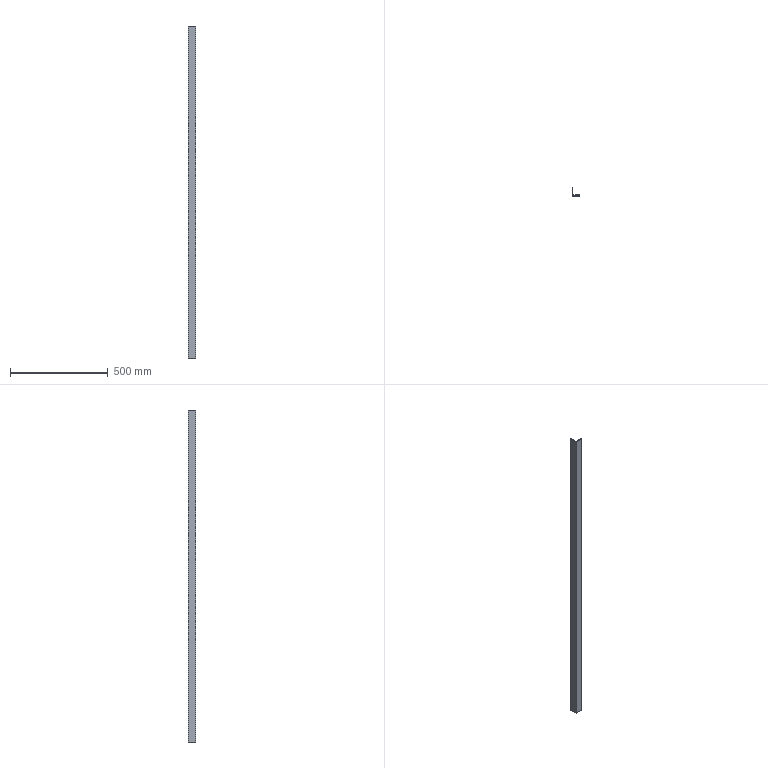Part | SolidWorks | features Extrusion 1 | 1 solid | 11 faces | box 40 x 40 x 1700 mm | volume 524623 mm3 | plane 8 | cylinder 3 | commonest cylinder face diameters 2.667 x2 10 x1
STEP:
#1=CARTESIAN_POINT('',(9.,4.,0.));
#2=VERTEX_POINT('',#1);
#3=CARTESIAN_POINT('',(4.,9.,0.));
#4=VERTEX_POINT('',#3);
#5=CARTESIAN_POINT('',(9.,9.,0.));
#6=DIRECTION('',(0.,0.,-1.));
#7=DIRECTION('',(-1.,0.,0.));
#8=AXIS2_PLACEMENT_3D('',#5,#6,#7);
#9=CIRCLE('',#8,5.);
#10=EDGE_CURVE('',#2,#4,#9,.T.);
#11=ORIENTED_EDGE('',*,*,#10,.T.);
#12=CARTESIAN_POINT('',(4.,9.,1700.));
#13=VERTEX_POINT('',#12);
#14=CARTESIAN_POINT('',(4.,9.,1700.));
#15=DIRECTION('',(0.,0.,-1.));
#16=VECTOR('',#15,1000.);
#17=LINE('',#14,#16);
#18=EDGE_CURVE('',#13,#4,#17,.T.);
#19=ORIENTED_EDGE('',*,*,#18,.F.);
#20=CARTESIAN_POINT('',(9.,4.,1700.));
#21=VERTEX_POINT('',#20);
#22=CARTESIAN_POINT('',(9.,9.,1700.));
#23=DIRECTION('',(0.,0.,-1.));
#24=DIRECTION('',(-1.,0.,0.));
#25=AXIS2_PLACEMENT_3D('',#22,#23,#24);
#26=CIRCLE('',#25,5.);
#27=EDGE_CURVE('',#21,#13,#26,.T.);
#28=ORIENTED_EDGE('',*,*,#27,.F.);
#29=CARTESIAN_POINT('',(9.,4.,1700.));
#30=DIRECTION('',(0.,0.,-1.));
#31=VECTOR('',#30,1000.);
#32=LINE('',#29,#31);
#33=EDGE_CURVE('',#21,#2,#32,.T.);
#34=ORIENTED_EDGE('',*,*,#33,.T.);
#35=EDGE_LOOP('',(#11,#19,#28,#34));
#36=FACE_OUTER_BOUND('',#35,.T.);
#37=CARTESIAN_POINT('',(9.,9.,1700.));
#38=DIRECTION('',(0.,0.,-1.));
#39=DIRECTION('',(-1.,0.,0.));
#40=AXIS2_PLACEMENT_3D('',#37,#38,#39);
#41=CYLINDRICAL_SURFACE('',#40,5.);
#42=ADVANCED_FACE('',(#36),#41,.F.);
#43=CARTESIAN_POINT('',(4.,38.667,0.));
#44=VERTEX_POINT('',#43);
#45=CARTESIAN_POINT('',(4.,38.667,0.));
#46=DIRECTION('',(0.,-1.,0.));
#47=VECTOR('',#46,1000.);
#48=LINE('',#45,#47);
#49=EDGE_CURVE('',#44,#4,#48,.T.);
#50=ORIENTED_EDGE('',*,*,#49,.F.);
#51=CARTESIAN_POINT('',(4.,38.667,1700.));
#52=VERTEX_POINT('',#51);
#53=CARTESIAN_POINT('',(4.,38.667,1700.));
#54=DIRECTION('',(0.,0.,-1.));
#55=VECTOR('',#54,1000.);
#56=LINE('',#53,#55);
#57=EDGE_CURVE('',#52,#44,#56,.T.);
#58=ORIENTED_EDGE('',*,*,#57,.F.);
#59=CARTESIAN_POINT('',(4.,38.667,1700.));
#60=DIRECTION('',(0.,-1.,0.));
#61=VECTOR('',#60,1000.);
#62=LINE('',#59,#61);
#63=EDGE_CURVE('',#52,#13,#62,.T.);
#64=ORIENTED_EDGE('',*,*,#63,.T.);
#65=ORIENTED_EDGE('',*,*,#18,.T.);
#66=EDGE_LOOP('',(#50,#58,#64,#65));
#67=FACE_OUTER_BOUND('',#66,.T.);
#68=CARTESIAN_POINT('',(4.,38.667,1700.));
#69=DIRECTION('',(1.,0.,0.));
#70=DIRECTION('',(0.,1.,0.));
#71=AXIS2_PLACEMENT_3D('',#68,#69,#70);
#72=PLANE('',#71);
#73=ADVANCED_FACE('',(#67),#72,.T.);
#74=CARTESIAN_POINT('',(2.667,40.,0.));
#75=VERTEX_POINT('',#74);
#76=CARTESIAN_POINT('',(2.667,38.667,0.));
#77=DIRECTION('',(0.,0.,-1.));
#78=DIRECTION('',(-1.,0.,0.));
#79=AXIS2_PLACEMENT_3D('',#76,#77,#78);
#80=CIRCLE('',#79,1.333);
#81=EDGE_CURVE('',#75,#44,#80,.T.);
#82=ORIENTED_EDGE('',*,*,#81,.F.);
#83=CARTESIAN_POINT('',(2.667,40.,1700.));
#84=VERTEX_POINT('',#83);
#85=CARTESIAN_POINT('',(2.667,40.,1700.));
#86=DIRECTION('',(0.,0.,-1.));
#87=VECTOR('',#86,1000.);
#88=LINE('',#85,#87);
#89=EDGE_CURVE('',#84,#75,#88,.T.);
#90=ORIENTED_EDGE('',*,*,#89,.F.);
#91=CARTESIAN_POINT('',(2.667,38.667,1700.));
#92=DIRECTION('',(0.,0.,-1.));
#93=DIRECTION('',(-1.,0.,0.));
#94=AXIS2_PLACEMENT_3D('',#91,#92,#93);
#95=CIRCLE('',#94,1.333);
#96=EDGE_CURVE('',#84,#52,#95,.T.);
#97=ORIENTED_EDGE('',*,*,#96,.T.);
#98=ORIENTED_EDGE('',*,*,#57,.T.);
#99=EDGE_LOOP('',(#82,#90,#97,#98));
#100=FACE_OUTER_BOUND('',#99,.T.);
#101=CARTESIAN_POINT('',(2.667,38.667,1700.));
#102=DIRECTION('',(0.,0.,-1.));
#103=DIRECTION('',(-1.,0.,0.));
#104=AXIS2_PLACEMENT_3D('',#101,#102,#103);
#105=CYLINDRICAL_SURFACE('',#104,1.333);
#106=ADVANCED_FACE('',(#100),#105,.T.);
#107=CARTESIAN_POINT('',(0.,40.,0.));
#108=VERTEX_POINT('',#107);
#109=CARTESIAN_POINT('',(0.,40.,0.));
#110=DIRECTION('',(1.,0.,0.));
#111=VECTOR('',#110,1000.);
#112=LINE('',#109,#111);
#113=EDGE_CURVE('',#108,#75,#112,.T.);
#114=ORIENTED_EDGE('',*,*,#113,.F.);
#115=CARTESIAN_POINT('',(0.,40.,1700.));
#116=VERTEX_POINT('',#115);
#117=CARTESIAN_POINT('',(0.,40.,1700.));
#118=DIRECTION('',(0.,0.,-1.));
#119=VECTOR('',#118,1000.);
#120=LINE('',#117,#119);
#121=EDGE_CURVE('',#116,#108,#120,.T.);
#122=ORIENTED_EDGE('',*,*,#121,.F.);
#123=CARTESIAN_POINT('',(0.,40.,1700.));
#124=DIRECTION('',(1.,0.,0.));
#125=VECTOR('',#124,1000.);
#126=LINE('',#123,#125);
#127=EDGE_CURVE('',#116,#84,#126,.T.);
#128=ORIENTED_EDGE('',*,*,#127,.T.);
#129=ORIENTED_EDGE('',*,*,#89,.T.);
#130=EDGE_LOOP('',(#114,#122,#128,#129));
#131=FACE_OUTER_BOUND('',#130,.T.);
#132=CARTESIAN_POINT('',(0.,40.,1700.));
#133=DIRECTION('',(0.,1.,0.));
#134=DIRECTION('',(0.,0.,1.));
#135=AXIS2_PLACEMENT_3D('',#132,#133,#134);
#136=PLANE('',#135);
#137=ADVANCED_FACE('',(#131),#136,.T.);
#138=CARTESIAN_POINT('',(0.,0.,0.));
#139=VERTEX_POINT('',#138);
#140=CARTESIAN_POINT('',(0.,0.,0.));
#141=DIRECTION('',(0.,1.,0.));
#142=VECTOR('',#141,1000.);
#143=LINE('',#140,#142);
#144=EDGE_CURVE('',#139,#108,#143,.T.);
#145=ORIENTED_EDGE('',*,*,#144,.F.);
#146=CARTESIAN_POINT('',(0.,0.,1700.));
#147=VERTEX_POINT('',#146);
#148=CARTESIAN_POINT('',(0.,0.,1700.));
#149=DIRECTION('',(0.,0.,-1.));
#150=VECTOR('',#149,1000.);
#151=LINE('',#148,#150);
#152=EDGE_CURVE('',#147,#139,#151,.T.);
#153=ORIENTED_EDGE('',*,*,#152,.F.);
#154=CARTESIAN_POINT('',(0.,0.,1700.));
#155=DIRECTION('',(0.,1.,0.));
#156=VECTOR('',#155,1000.);
#157=LINE('',#154,#156);
#158=EDGE_CURVE('',#147,#116,#157,.T.);
#159=ORIENTED_EDGE('',*,*,#158,.T.);
#160=ORIENTED_EDGE('',*,*,#121,.T.);
#161=EDGE_LOOP('',(#145,#153,#159,#160));
#162=FACE_OUTER_BOUND('',#161,.T.);
#163=CARTESIAN_POINT('',(0.,0.,1700.));
#164=DIRECTION('',(-1.,0.,0.));
#165=DIRECTION('',(0.,0.,1.));
#166=AXIS2_PLACEMENT_3D('',#163,#164,#165);
#167=PLANE('',#166);
#168=ADVANCED_FACE('',(#162),#167,.T.);
#169=CARTESIAN_POINT('',(40.,0.,0.));
#170=VERTEX_POINT('',#169);
#171=CARTESIAN_POINT('',(40.,0.,0.));
#172=DIRECTION('',(-1.,0.,0.));
#173=VECTOR('',#172,1000.);
#174=LINE('',#171,#173);
#175=EDGE_CURVE('',#170,#139,#174,.T.);
#176=ORIENTED_EDGE('',*,*,#175,.F.);
#177=CARTESIAN_POINT('',(40.,0.,1700.));
#178=VERTEX_POINT('',#177);
#179=CARTESIAN_POINT('',(40.,0.,1700.));
#180=DIRECTION('',(0.,0.,-1.));
#181=VECTOR('',#180,1000.);
#182=LINE('',#179,#181);
#183=EDGE_CURVE('',#178,#170,#182,.T.);
#184=ORIENTED_EDGE('',*,*,#183,.F.);
#185=CARTESIAN_POINT('',(40.,0.,1700.));
#186=DIRECTION('',(-1.,0.,0.));
#187=VECTOR('',#186,1000.);
#188=LINE('',#185,#187);
#189=EDGE_CURVE('',#178,#147,#188,.T.);
#190=ORIENTED_EDGE('',*,*,#189,.T.);
#191=ORIENTED_EDGE('',*,*,#152,.T.);
#192=EDGE_LOOP('',(#176,#184,#190,#191));
#193=FACE_OUTER_BOUND('',#192,.T.);
#194=CARTESIAN_POINT('',(40.,0.,1700.));
#195=DIRECTION('',(0.,-1.,0.));
#196=DIRECTION('',(0.,0.,-1.));
#197=AXIS2_PLACEMENT_3D('',#194,#195,#196);
#198=PLANE('',#197);
#199=ADVANCED_FACE('',(#193),#198,.T.);
#200=CARTESIAN_POINT('',(40.,2.667,0.));
#201=VERTEX_POINT('',#200);
#202=CARTESIAN_POINT('',(40.,0.,0.));
#203=DIRECTION('',(0.,1.,0.));
#204=VECTOR('',#203,1000.);
#205=LINE('',#202,#204);
#206=EDGE_CURVE('',#170,#201,#205,.T.);
#207=ORIENTED_EDGE('',*,*,#206,.T.);
#208=CARTESIAN_POINT('',(40.,2.667,1700.));
#209=VERTEX_POINT('',#208);
#210=CARTESIAN_POINT('',(40.,2.667,1700.));
#211=DIRECTION('',(0.,0.,-1.));
#212=VECTOR('',#211,1000.);
#213=LINE('',#210,#212);
#214=EDGE_CURVE('',#209,#201,#213,.T.);
#215=ORIENTED_EDGE('',*,*,#214,.F.);
#216=CARTESIAN_POINT('',(40.,0.,1700.));
#217=DIRECTION('',(0.,1.,0.));
#218=VECTOR('',#217,1000.);
#219=LINE('',#216,#218);
#220=EDGE_CURVE('',#178,#209,#219,.T.);
#221=ORIENTED_EDGE('',*,*,#220,.F.);
#222=ORIENTED_EDGE('',*,*,#183,.T.);
#223=EDGE_LOOP('',(#207,#215,#221,#222));
#224=FACE_OUTER_BOUND('',#223,.T.);
#225=CARTESIAN_POINT('',(40.,0.,1700.));
#226=DIRECTION('',(-1.,0.,0.));
#227=DIRECTION('',(0.,-1.,0.));
#228=AXIS2_PLACEMENT_3D('',#225,#226,#227);
#229=PLANE('',#228);
#230=ADVANCED_FACE('',(#224),#229,.F.);
#231=CARTESIAN_POINT('',(38.667,4.,0.));
#232=VERTEX_POINT('',#231);
#233=CARTESIAN_POINT('',(38.667,2.667,0.));
#234=DIRECTION('',(0.,0.,1.));
#235=DIRECTION('',(1.,0.,0.));
#236=AXIS2_PLACEMENT_3D('',#233,#234,#235);
#237=CIRCLE('',#236,1.333);
#238=EDGE_CURVE('',#201,#232,#237,.T.);
#239=ORIENTED_EDGE('',*,*,#238,.T.);
#240=CARTESIAN_POINT('',(38.667,4.,1700.));
#241=VERTEX_POINT('',#240);
#242=CARTESIAN_POINT('',(38.667,4.,1700.));
#243=DIRECTION('',(0.,0.,-1.));
#244=VECTOR('',#243,1000.);
#245=LINE('',#242,#244);
#246=EDGE_CURVE('',#241,#232,#245,.T.);
#247=ORIENTED_EDGE('',*,*,#246,.F.);
#248=CARTESIAN_POINT('',(38.667,2.667,1700.));
#249=DIRECTION('',(0.,0.,1.));
#250=DIRECTION('',(1.,0.,0.));
#251=AXIS2_PLACEMENT_3D('',#248,#249,#250);
#252=CIRCLE('',#251,1.333);
#253=EDGE_CURVE('',#209,#241,#252,.T.);
#254=ORIENTED_EDGE('',*,*,#253,.F.);
#255=ORIENTED_EDGE('',*,*,#214,.T.);
#256=EDGE_LOOP('',(#239,#247,#254,#255));
#257=FACE_OUTER_BOUND('',#256,.T.);
#258=CARTESIAN_POINT('',(38.667,2.667,1700.));
#259=DIRECTION('',(0.,0.,-1.));
#260=DIRECTION('',(-1.,0.,0.));
#261=AXIS2_PLACEMENT_3D('',#258,#259,#260);
#262=CYLINDRICAL_SURFACE('',#261,1.333);
#263=ADVANCED_FACE('',(#257),#262,.T.);
#264=CARTESIAN_POINT('',(9.,4.,0.));
#265=DIRECTION('',(1.,0.,0.));
#266=VECTOR('',#265,1000.);
#267=LINE('',#264,#266);
#268=EDGE_CURVE('',#2,#232,#267,.T.);
#269=ORIENTED_EDGE('',*,*,#268,.F.);
#270=ORIENTED_EDGE('',*,*,#33,.F.);
#271=CARTESIAN_POINT('',(9.,4.,1700.));
#272=DIRECTION('',(1.,0.,0.));
#273=VECTOR('',#272,1000.);
#274=LINE('',#271,#273);
#275=EDGE_CURVE('',#21,#241,#274,.T.);
#276=ORIENTED_EDGE('',*,*,#275,.T.);
#277=ORIENTED_EDGE('',*,*,#246,.T.);
#278=EDGE_LOOP('',(#269,#270,#276,#277));
#279=FACE_OUTER_BOUND('',#278,.T.);
#280=CARTESIAN_POINT('',(9.,4.,1700.));
#281=DIRECTION('',(0.,1.,0.));
#282=DIRECTION('',(-1.,0.,0.));
#283=AXIS2_PLACEMENT_3D('',#280,#281,#282);
#284=PLANE('',#283);
#285=ADVANCED_FACE('',(#279),#284,.T.);
#286=ORIENTED_EDGE('',*,*,#27,.T.);
#287=ORIENTED_EDGE('',*,*,#63,.F.);
#288=ORIENTED_EDGE('',*,*,#96,.F.);
#289=ORIENTED_EDGE('',*,*,#127,.F.);
#290=ORIENTED_EDGE('',*,*,#158,.F.);
#291=ORIENTED_EDGE('',*,*,#189,.F.);
#292=ORIENTED_EDGE('',*,*,#220,.T.);
#293=ORIENTED_EDGE('',*,*,#253,.T.);
#294=ORIENTED_EDGE('',*,*,#275,.F.);
#295=EDGE_LOOP('',(#286,#287,#288,#289,#290,#291,#292,#293,#294));
#296=FACE_OUTER_BOUND('',#295,.T.);
#297=CARTESIAN_POINT('',(9.,9.,1700.));
#298=DIRECTION('',(0.,0.,-1.));
#299=DIRECTION('',(-1.,0.,0.));
#300=AXIS2_PLACEMENT_3D('',#297,#298,#299);
#301=PLANE('',#300);
#302=ADVANCED_FACE('',(#296),#301,.F.);
#303=ORIENTED_EDGE('',*,*,#10,.F.);
#304=ORIENTED_EDGE('',*,*,#268,.T.);
#305=ORIENTED_EDGE('',*,*,#238,.F.);
#306=ORIENTED_EDGE('',*,*,#206,.F.);
#307=ORIENTED_EDGE('',*,*,#175,.T.);
#308=ORIENTED_EDGE('',*,*,#144,.T.);
#309=ORIENTED_EDGE('',*,*,#113,.T.);
#310=ORIENTED_EDGE('',*,*,#81,.T.);
#311=ORIENTED_EDGE('',*,*,#49,.T.);
#312=EDGE_LOOP('',(#303,#304,#305,#306,#307,#308,#309,#310,#311));
#313=FACE_OUTER_BOUND('',#312,.T.);
#314=CARTESIAN_POINT('',(9.,9.,0.));
#315=DIRECTION('',(0.,0.,-1.));
#316=DIRECTION('',(-1.,0.,0.));
#317=AXIS2_PLACEMENT_3D('',#314,#315,#316);
#318=PLANE('',#317);
#319=ADVANCED_FACE('',(#313),#318,.T.);
#320=CLOSED_SHELL('',(#42,#73,#106,#137,#168,#199,#230,#263,#285,#302,#319));
#321=MANIFOLD_SOLID_BREP('',#320);
#322=CARTESIAN_POINT('',(0.,0.,0.));
#323=DIRECTION('',(0.,0.,1.));
#324=DIRECTION('',(1.,0.,0.));
#325=AXIS2_PLACEMENT_3D('',#322,#323,#324);
#326=(LENGTH_UNIT()NAMED_UNIT(*)SI_UNIT(.MILLI.,.METRE.));
#327=UNCERTAINTY_MEASURE_WITH_UNIT(LENGTH_MEASURE(0.00001),#326,'','');
#328=(NAMED_UNIT(*)PLANE_ANGLE_UNIT()SI_UNIT($,.RADIAN.));
#329=(NAMED_UNIT(*)SI_UNIT($,.STERADIAN.)SOLID_ANGLE_UNIT());
#330=(GEOMETRIC_REPRESENTATION_CONTEXT(3)GLOBAL_UNCERTAINTY_ASSIGNED_CONTEXT((#327))GLOBAL_UNIT_ASSIGNED_CONTEXT((#326,#328,#329))REPRESENTATION_CONTEXT('',''));
#331=ADVANCED_BREP_SHAPE_REPRESENTATION('',(#321,#325),#330);